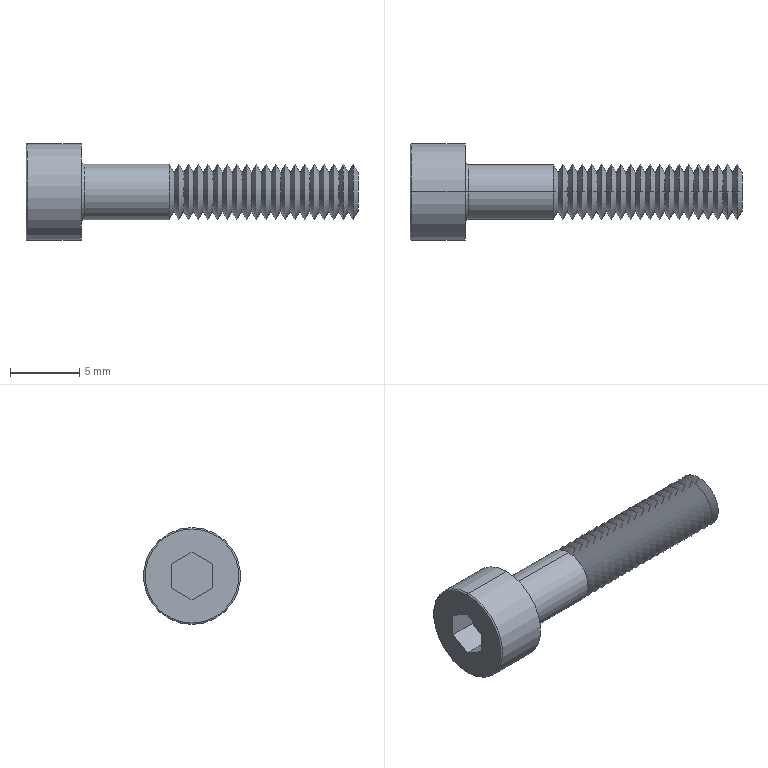Part | SolidWorks | features BlendCut 1, Cut 1, Fillet 1, LPattern 1, RevCut 1, Revolution 1 | 1 solid | 134 faces | box 24 x 7 x 7 mm | volume 343.22 mm3 | cone 78 | cylinder 42 | plane 10 | torus 4 | commonest cylinder face diameters 4 x40 7 x2